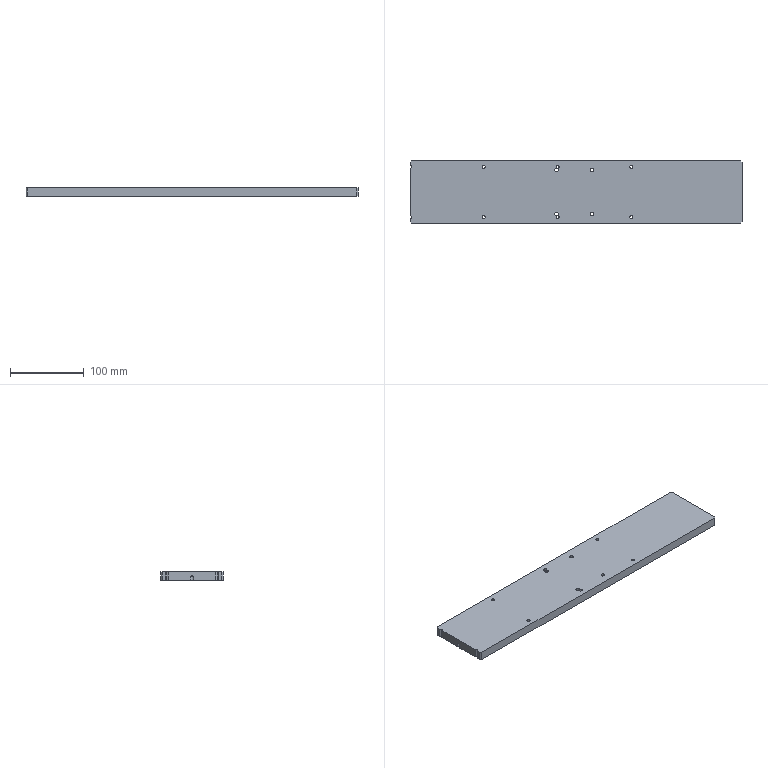Part | SolidWorks | features BaseBody 1 | 1 solid | 46 faces | box 450 x 85 x 12 mm | volume 456645 mm3 | cylinder 31 | plane 12 | cone 3 | commonest cylinder face diameters 4.2 x18 5 x13
STEP:
#1=CARTESIAN_POINT('',(-225.,-40.5,12.));
#2=VERTEX_POINT('',#1);
#3=CARTESIAN_POINT('',(-223.,-42.5,12.));
#4=VERTEX_POINT('',#3);
#5=CARTESIAN_POINT('',(-223.,-42.5,12.));
#6=DIRECTION('',(0.7071,-0.7071,0.));
#7=VECTOR('',#6,1000.);
#8=LINE('',#5,#7);
#9=EDGE_CURVE('',#2,#4,#8,.T.);
#10=ORIENTED_EDGE('',*,*,#9,.F.);
#11=CARTESIAN_POINT('',(-225.,-40.5,0.));
#12=VERTEX_POINT('',#11);
#13=CARTESIAN_POINT('',(-225.,-40.5,12.));
#14=DIRECTION('',(0.,0.,1.));
#15=VECTOR('',#14,1000.);
#16=LINE('',#13,#15);
#17=EDGE_CURVE('',#12,#2,#16,.T.);
#18=ORIENTED_EDGE('',*,*,#17,.F.);
#19=CARTESIAN_POINT('',(-223.,-42.5,0.));
#20=VERTEX_POINT('',#19);
#21=CARTESIAN_POINT('',(-132.75,-132.75,0.));
#22=DIRECTION('',(-0.7071,0.7071,0.));
#23=VECTOR('',#22,1000.);
#24=LINE('',#21,#23);
#25=EDGE_CURVE('',#20,#12,#24,.T.);
#26=ORIENTED_EDGE('',*,*,#25,.F.);
#27=CARTESIAN_POINT('',(-223.,-42.5,12.));
#28=DIRECTION('',(0.,0.,-1.));
#29=VECTOR('',#28,1000.);
#30=LINE('',#27,#29);
#31=EDGE_CURVE('',#4,#20,#30,.T.);
#32=ORIENTED_EDGE('',*,*,#31,.F.);
#33=EDGE_LOOP('',(#10,#18,#26,#32));
#34=FACE_OUTER_BOUND('',#33,.T.);
#35=CARTESIAN_POINT('',(-223.,-42.5,12.));
#36=DIRECTION('',(0.7071,0.7071,0.));
#37=DIRECTION('',(0.,0.,-1.));
#38=AXIS2_PLACEMENT_3D('',#35,#36,#37);
#39=PLANE('',#38);
#40=ADVANCED_FACE('',(#34),#39,.F.);
#41=CARTESIAN_POINT('',(-223.,42.5,12.));
#42=VERTEX_POINT('',#41);
#43=CARTESIAN_POINT('',(-225.,40.5,12.));
#44=VERTEX_POINT('',#43);
#45=CARTESIAN_POINT('',(-225.,40.5,12.));
#46=DIRECTION('',(-0.7071,-0.7071,0.));
#47=VECTOR('',#46,1000.);
#48=LINE('',#45,#47);
#49=EDGE_CURVE('',#42,#44,#48,.T.);
#50=ORIENTED_EDGE('',*,*,#49,.F.);
#51=CARTESIAN_POINT('',(-223.,42.5,0.));
#52=VERTEX_POINT('',#51);
#53=CARTESIAN_POINT('',(-223.,42.5,12.));
#54=DIRECTION('',(0.,0.,1.));
#55=VECTOR('',#54,1000.);
#56=LINE('',#53,#55);
#57=EDGE_CURVE('',#52,#42,#56,.T.);
#58=ORIENTED_EDGE('',*,*,#57,.F.);
#59=CARTESIAN_POINT('',(-225.,40.5,0.));
#60=VERTEX_POINT('',#59);
#61=CARTESIAN_POINT('',(-132.75,132.75,0.));
#62=DIRECTION('',(0.7071,0.7071,0.));
#63=VECTOR('',#62,1000.);
#64=LINE('',#61,#63);
#65=EDGE_CURVE('',#60,#52,#64,.T.);
#66=ORIENTED_EDGE('',*,*,#65,.F.);
#67=CARTESIAN_POINT('',(-225.,40.5,12.));
#68=DIRECTION('',(0.,0.,-1.));
#69=VECTOR('',#68,1000.);
#70=LINE('',#67,#69);
#71=EDGE_CURVE('',#44,#60,#70,.T.);
#72=ORIENTED_EDGE('',*,*,#71,.F.);
#73=EDGE_LOOP('',(#50,#58,#66,#72));
#74=FACE_OUTER_BOUND('',#73,.T.);
#75=CARTESIAN_POINT('',(-225.,40.5,12.));
#76=DIRECTION('',(0.7071,-0.7071,0.));
#77=DIRECTION('',(0.,0.,-1.));
#78=AXIS2_PLACEMENT_3D('',#75,#76,#77);
#79=PLANE('',#78);
#80=ADVANCED_FACE('',(#74),#79,.F.);
#81=CARTESIAN_POINT('',(223.,-42.5,12.));
#82=VERTEX_POINT('',#81);
#83=CARTESIAN_POINT('',(225.,-40.5,12.));
#84=VERTEX_POINT('',#83);
#85=CARTESIAN_POINT('',(225.,-40.5,12.));
#86=DIRECTION('',(0.7071,0.7071,0.));
#87=VECTOR('',#86,1000.);
#88=LINE('',#85,#87);
#89=EDGE_CURVE('',#82,#84,#88,.T.);
#90=ORIENTED_EDGE('',*,*,#89,.F.);
#91=CARTESIAN_POINT('',(223.,-42.5,0.));
#92=VERTEX_POINT('',#91);
#93=CARTESIAN_POINT('',(223.,-42.5,12.));
#94=DIRECTION('',(0.,0.,1.));
#95=VECTOR('',#94,1000.);
#96=LINE('',#93,#95);
#97=EDGE_CURVE('',#92,#82,#96,.T.);
#98=ORIENTED_EDGE('',*,*,#97,.F.);
#99=CARTESIAN_POINT('',(225.,-40.5,0.));
#100=VERTEX_POINT('',#99);
#101=CARTESIAN_POINT('',(132.75,-132.75,0.));
#102=DIRECTION('',(-0.7071,-0.7071,0.));
#103=VECTOR('',#102,1000.);
#104=LINE('',#101,#103);
#105=EDGE_CURVE('',#100,#92,#104,.T.);
#106=ORIENTED_EDGE('',*,*,#105,.F.);
#107=CARTESIAN_POINT('',(225.,-40.5,12.));
#108=DIRECTION('',(0.,0.,-1.));
#109=VECTOR('',#108,1000.);
#110=LINE('',#107,#109);
#111=EDGE_CURVE('',#84,#100,#110,.T.);
#112=ORIENTED_EDGE('',*,*,#111,.F.);
#113=EDGE_LOOP('',(#90,#98,#106,#112));
#114=FACE_OUTER_BOUND('',#113,.T.);
#115=CARTESIAN_POINT('',(225.,-40.5,12.));
#116=DIRECTION('',(-0.7071,0.7071,0.));
#117=DIRECTION('',(0.,0.,1.));
#118=AXIS2_PLACEMENT_3D('',#115,#116,#117);
#119=PLANE('',#118);
#120=ADVANCED_FACE('',(#114),#119,.F.);
#121=CARTESIAN_POINT('',(225.,40.5,12.));
#122=VERTEX_POINT('',#121);
#123=CARTESIAN_POINT('',(223.,42.5,12.));
#124=VERTEX_POINT('',#123);
#125=CARTESIAN_POINT('',(223.,42.5,12.));
#126=DIRECTION('',(-0.7071,0.7071,0.));
#127=VECTOR('',#126,1000.);
#128=LINE('',#125,#127);
#129=EDGE_CURVE('',#122,#124,#128,.T.);
#130=ORIENTED_EDGE('',*,*,#129,.F.);
#131=CARTESIAN_POINT('',(225.,40.5,0.));
#132=VERTEX_POINT('',#131);
#133=CARTESIAN_POINT('',(225.,40.5,12.));
#134=DIRECTION('',(0.,0.,1.));
#135=VECTOR('',#134,1000.);
#136=LINE('',#133,#135);
#137=EDGE_CURVE('',#132,#122,#136,.T.);
#138=ORIENTED_EDGE('',*,*,#137,.F.);
#139=CARTESIAN_POINT('',(223.,42.5,0.));
#140=VERTEX_POINT('',#139);
#141=CARTESIAN_POINT('',(132.75,132.75,0.));
#142=DIRECTION('',(0.7071,-0.7071,0.));
#143=VECTOR('',#142,1000.);
#144=LINE('',#141,#143);
#145=EDGE_CURVE('',#140,#132,#144,.T.);
#146=ORIENTED_EDGE('',*,*,#145,.F.);
#147=CARTESIAN_POINT('',(223.,42.5,12.));
#148=DIRECTION('',(0.,0.,-1.));
#149=VECTOR('',#148,1000.);
#150=LINE('',#147,#149);
#151=EDGE_CURVE('',#124,#140,#150,.T.);
#152=ORIENTED_EDGE('',*,*,#151,.F.);
#153=EDGE_LOOP('',(#130,#138,#146,#152));
#154=FACE_OUTER_BOUND('',#153,.T.);
#155=CARTESIAN_POINT('',(223.,42.5,12.));
#156=DIRECTION('',(-0.7071,-0.7071,0.));
#157=DIRECTION('',(-0.7071,0.7071,0.));
#158=AXIS2_PLACEMENT_3D('',#155,#156,#157);
#159=PLANE('',#158);
#160=ADVANCED_FACE('',(#154),#159,.F.);
#161=CARTESIAN_POINT('',(77.5,0.,5.));
#162=VERTEX_POINT('',#161);
#163=CARTESIAN_POINT('',(77.5,0.,0.));
#164=VERTEX_POINT('',#163);
#165=CARTESIAN_POINT('',(77.5,0.,0.));
#166=DIRECTION('',(0.,0.,-1.));
#167=VECTOR('',#166,1000.);
#168=LINE('',#165,#167);
#169=EDGE_CURVE('',#162,#164,#168,.T.);
#170=ORIENTED_EDGE('',*,*,#169,.F.);
#171=CARTESIAN_POINT('',(72.5,0.,5.));
#172=VERTEX_POINT('',#171);
#173=CARTESIAN_POINT('',(75.,0.,5.));
#174=DIRECTION('',(0.,0.,-1.));
#175=DIRECTION('',(-1.,0.,0.));
#176=AXIS2_PLACEMENT_3D('',#173,#174,#175);
#177=CIRCLE('',#176,2.5);
#178=EDGE_CURVE('',#172,#162,#177,.T.);
#179=ORIENTED_EDGE('',*,*,#178,.F.);
#180=CARTESIAN_POINT('',(72.5,0.,0.));
#181=VERTEX_POINT('',#180);
#182=CARTESIAN_POINT('',(72.5,0.,0.));
#183=DIRECTION('',(0.,0.,-1.));
#184=VECTOR('',#183,1000.);
#185=LINE('',#182,#184);
#186=EDGE_CURVE('',#172,#181,#185,.T.);
#187=ORIENTED_EDGE('',*,*,#186,.T.);
#188=CARTESIAN_POINT('',(75.,0.,0.));
#189=DIRECTION('',(0.,0.,-1.));
#190=DIRECTION('',(-1.,0.,0.));
#191=AXIS2_PLACEMENT_3D('',#188,#189,#190);
#192=CIRCLE('',#191,2.5);
#193=EDGE_CURVE('',#181,#164,#192,.T.);
#194=ORIENTED_EDGE('',*,*,#193,.T.);
#195=EDGE_LOOP('',(#170,#179,#187,#194));
#196=FACE_OUTER_BOUND('',#195,.T.);
#197=CARTESIAN_POINT('',(75.,0.,0.));
#198=DIRECTION('',(0.,0.,-1.));
#199=DIRECTION('',(-1.,0.,0.));
#200=AXIS2_PLACEMENT_3D('',#197,#198,#199);
#201=CYLINDRICAL_SURFACE('',#200,2.5);
#202=ADVANCED_FACE('',(#196),#201,.F.);
#203=CARTESIAN_POINT('',(75.,0.,6.502));
#204=VERTEX_POINT('',#203);
#205=CARTESIAN_POINT('',(77.5,0.,5.));
#206=DIRECTION('',(0.8572,0.,-0.515));
#207=VECTOR('',#206,1000.);
#208=LINE('',#205,#207);
#209=EDGE_CURVE('',#204,#162,#208,.T.);
#210=ORIENTED_EDGE('',*,*,#209,.F.);
#211=CARTESIAN_POINT('',(72.5,0.,5.));
#212=DIRECTION('',(-0.8572,0.,-0.515));
#213=VECTOR('',#212,1000.);
#214=LINE('',#211,#213);
#215=EDGE_CURVE('',#204,#172,#214,.T.);
#216=ORIENTED_EDGE('',*,*,#215,.T.);
#217=ORIENTED_EDGE('',*,*,#178,.T.);
#218=EDGE_LOOP('',(#210,#216,#217));
#219=FACE_OUTER_BOUND('',#218,.T.);
#220=CARTESIAN_POINT('',(75.,0.,5.));
#221=DIRECTION('',(0.,0.,-1.));
#222=DIRECTION('',(-1.,0.,0.));
#223=AXIS2_PLACEMENT_3D('',#220,#221,#222);
#224=CONICAL_SURFACE('',#223,2.5,1.03);
#225=ADVANCED_FACE('',(#219),#224,.F.);
#226=CARTESIAN_POINT('',(-225.,2.5,5.));
#227=VERTEX_POINT('',#226);
#228=CARTESIAN_POINT('',(-225.,0.,6.502));
#229=VERTEX_POINT('',#228);
#230=CARTESIAN_POINT('',(-225.,0.,6.502));
#231=DIRECTION('',(0.,-0.8572,0.515));
#232=VECTOR('',#231,1000.);
#233=LINE('',#230,#232);
#234=EDGE_CURVE('',#227,#229,#233,.T.);
#235=ORIENTED_EDGE('',*,*,#234,.F.);
#236=CARTESIAN_POINT('',(-225.,-2.5,5.));
#237=VERTEX_POINT('',#236);
#238=CARTESIAN_POINT('',(-225.,0.,5.));
#239=DIRECTION('',(0.,0.,-1.));
#240=DIRECTION('',(-1.,0.,0.));
#241=AXIS2_PLACEMENT_3D('',#238,#239,#240);
#242=CIRCLE('',#241,2.5);
#243=EDGE_CURVE('',#227,#237,#242,.T.);
#244=ORIENTED_EDGE('',*,*,#243,.T.);
#245=CARTESIAN_POINT('',(-225.,0.,6.502));
#246=DIRECTION('',(0.,-0.8572,-0.515));
#247=VECTOR('',#246,1000.);
#248=LINE('',#245,#247);
#249=EDGE_CURVE('',#229,#237,#248,.T.);
#250=ORIENTED_EDGE('',*,*,#249,.F.);
#251=EDGE_LOOP('',(#235,#244,#250));
#252=FACE_OUTER_BOUND('',#251,.T.);
#253=CARTESIAN_POINT('',(-225.,0.,5.));
#254=DIRECTION('',(0.,0.,-1.));
#255=DIRECTION('',(-1.,0.,0.));
#256=AXIS2_PLACEMENT_3D('',#253,#254,#255);
#257=CONICAL_SURFACE('',#256,2.5,1.03);
#258=ADVANCED_FACE('',(#252),#257,.F.);
#259=ORIENTED_EDGE('',*,*,#243,.F.);
#260=CARTESIAN_POINT('',(-225.,2.5,0.));
#261=VERTEX_POINT('',#260);
#262=CARTESIAN_POINT('',(-225.,2.5,0.));
#263=DIRECTION('',(0.,0.,1.));
#264=VECTOR('',#263,1000.);
#265=LINE('',#262,#264);
#266=EDGE_CURVE('',#261,#227,#265,.T.);
#267=ORIENTED_EDGE('',*,*,#266,.F.);
#268=CARTESIAN_POINT('',(-225.,-2.5,0.));
#269=VERTEX_POINT('',#268);
#270=CARTESIAN_POINT('',(-225.,0.,0.));
#271=DIRECTION('',(0.,0.,-1.));
#272=DIRECTION('',(-1.,0.,0.));
#273=AXIS2_PLACEMENT_3D('',#270,#271,#272);
#274=CIRCLE('',#273,2.5);
#275=EDGE_CURVE('',#261,#269,#274,.T.);
#276=ORIENTED_EDGE('',*,*,#275,.T.);
#277=CARTESIAN_POINT('',(-225.,-2.5,0.));
#278=DIRECTION('',(0.,0.,-1.));
#279=VECTOR('',#278,1000.);
#280=LINE('',#277,#279);
#281=EDGE_CURVE('',#237,#269,#280,.T.);
#282=ORIENTED_EDGE('',*,*,#281,.F.);
#283=EDGE_LOOP('',(#259,#267,#276,#282));
#284=FACE_OUTER_BOUND('',#283,.T.);
#285=CARTESIAN_POINT('',(-225.,0.,0.));
#286=DIRECTION('',(0.,0.,-1.));
#287=DIRECTION('',(-1.,0.,0.));
#288=AXIS2_PLACEMENT_3D('',#285,#286,#287);
#289=CYLINDRICAL_SURFACE('',#288,2.5);
#290=ADVANCED_FACE('',(#284),#289,.F.);
#291=CARTESIAN_POINT('',(72.9,34.,0.));
#292=VERTEX_POINT('',#291);
#293=CARTESIAN_POINT('',(72.9,34.,12.));
#294=VERTEX_POINT('',#293);
#295=CARTESIAN_POINT('',(72.9,34.,12.));
#296=DIRECTION('',(0.,0.,1.));
#297=VECTOR('',#296,1000.);
#298=LINE('',#295,#297);
#299=EDGE_CURVE('',#292,#294,#298,.T.);
#300=ORIENTED_EDGE('',*,*,#299,.F.);
#301=CARTESIAN_POINT('',(77.1,34.,0.));
#302=VERTEX_POINT('',#301);
#303=CARTESIAN_POINT('',(75.,34.,0.));
#304=DIRECTION('',(0.,0.,1.));
#305=DIRECTION('',(1.,0.,0.));
#306=AXIS2_PLACEMENT_3D('',#303,#304,#305);
#307=CIRCLE('',#306,2.1);
#308=EDGE_CURVE('',#302,#292,#307,.T.);
#309=ORIENTED_EDGE('',*,*,#308,.F.);
#310=CARTESIAN_POINT('',(77.1,34.,12.));
#311=VERTEX_POINT('',#310);
#312=CARTESIAN_POINT('',(77.1,34.,12.));
#313=DIRECTION('',(0.,0.,1.));
#314=VECTOR('',#313,1000.);
#315=LINE('',#312,#314);
#316=EDGE_CURVE('',#302,#311,#315,.T.);
#317=ORIENTED_EDGE('',*,*,#316,.T.);
#318=CARTESIAN_POINT('',(75.,34.,12.));
#319=DIRECTION('',(0.,0.,1.));
#320=DIRECTION('',(1.,0.,0.));
#321=AXIS2_PLACEMENT_3D('',#318,#319,#320);
#322=CIRCLE('',#321,2.1);
#323=EDGE_CURVE('',#311,#294,#322,.T.);
#324=ORIENTED_EDGE('',*,*,#323,.T.);
#325=EDGE_LOOP('',(#300,#309,#317,#324));
#326=FACE_OUTER_BOUND('',#325,.T.);
#327=CARTESIAN_POINT('',(75.,34.,12.));
#328=DIRECTION('',(0.,0.,1.));
#329=DIRECTION('',(1.,0.,0.));
#330=AXIS2_PLACEMENT_3D('',#327,#328,#329);
#331=CYLINDRICAL_SURFACE('',#330,2.1);
#332=ADVANCED_FACE('',(#326),#331,.F.);
#333=CARTESIAN_POINT('',(72.9,-34.,0.));
#334=VERTEX_POINT('',#333);
#335=CARTESIAN_POINT('',(72.9,-34.,12.));
#336=VERTEX_POINT('',#335);
#337=CARTESIAN_POINT('',(72.9,-34.,12.));
#338=DIRECTION('',(0.,0.,1.));
#339=VECTOR('',#338,1000.);
#340=LINE('',#337,#339);
#341=EDGE_CURVE('',#334,#336,#340,.T.);
#342=ORIENTED_EDGE('',*,*,#341,.F.);
#343=CARTESIAN_POINT('',(77.1,-34.,0.));
#344=VERTEX_POINT('',#343);
#345=CARTESIAN_POINT('',(75.,-34.,0.));
#346=DIRECTION('',(0.,0.,1.));
#347=DIRECTION('',(1.,0.,0.));
#348=AXIS2_PLACEMENT_3D('',#345,#346,#347);
#349=CIRCLE('',#348,2.1);
#350=EDGE_CURVE('',#344,#334,#349,.T.);
#351=ORIENTED_EDGE('',*,*,#350,.F.);
#352=CARTESIAN_POINT('',(77.1,-34.,12.));
#353=VERTEX_POINT('',#352);
#354=CARTESIAN_POINT('',(77.1,-34.,12.));
#355=DIRECTION('',(0.,0.,1.));
#356=VECTOR('',#355,1000.);
#357=LINE('',#354,#356);
#358=EDGE_CURVE('',#344,#353,#357,.T.);
#359=ORIENTED_EDGE('',*,*,#358,.T.);
#360=CARTESIAN_POINT('',(75.,-34.,12.));
#361=DIRECTION('',(0.,0.,1.));
#362=DIRECTION('',(1.,0.,0.));
#363=AXIS2_PLACEMENT_3D('',#360,#361,#362);
#364=CIRCLE('',#363,2.1);
#365=EDGE_CURVE('',#353,#336,#364,.T.);
#366=ORIENTED_EDGE('',*,*,#365,.T.);
#367=EDGE_LOOP('',(#342,#351,#359,#366));
#368=FACE_OUTER_BOUND('',#367,.T.);
#369=CARTESIAN_POINT('',(75.,-34.,12.));
#370=DIRECTION('',(0.,0.,1.));
#371=DIRECTION('',(1.,0.,0.));
#372=AXIS2_PLACEMENT_3D('',#369,#370,#371);
#373=CYLINDRICAL_SURFACE('',#372,2.1);
#374=ADVANCED_FACE('',(#368),#373,.F.);
#375=CARTESIAN_POINT('',(-22.9,34.,0.));
#376=VERTEX_POINT('',#375);
#377=CARTESIAN_POINT('',(-22.9,34.,12.));
#378=VERTEX_POINT('',#377);
#379=CARTESIAN_POINT('',(-22.9,34.,12.));
#380=DIRECTION('',(0.,0.,1.));
#381=VECTOR('',#380,1000.);
#382=LINE('',#379,#381);
#383=EDGE_CURVE('',#376,#378,#382,.T.);
#384=ORIENTED_EDGE('',*,*,#383,.F.);
#385=CARTESIAN_POINT('',(-24.879,31.903,0.));
#386=VERTEX_POINT('',#385);
#387=CARTESIAN_POINT('',(-25.,34.,0.));
#388=DIRECTION('',(0.,0.,-1.));
#389=DIRECTION('',(-1.,0.,0.));
#390=AXIS2_PLACEMENT_3D('',#387,#388,#389);
#391=CIRCLE('',#390,2.1);
#392=EDGE_CURVE('',#376,#386,#391,.T.);
#393=ORIENTED_EDGE('',*,*,#392,.T.);
#394=CARTESIAN_POINT('',(-24.879,31.903,12.));
#395=VERTEX_POINT('',#394);
#396=CARTESIAN_POINT('',(-24.879,31.903,6.));
#397=DIRECTION('',(0.,0.,-1.));
#398=VECTOR('',#397,1000.);
#399=LINE('',#396,#398);
#400=EDGE_CURVE('',#395,#386,#399,.T.);
#401=ORIENTED_EDGE('',*,*,#400,.F.);
#402=CARTESIAN_POINT('',(-25.,34.,12.));
#403=DIRECTION('',(0.,0.,1.));
#404=DIRECTION('',(1.,0.,0.));
#405=AXIS2_PLACEMENT_3D('',#402,#403,#404);
#406=CIRCLE('',#405,2.1);
#407=EDGE_CURVE('',#395,#378,#406,.T.);
#408=ORIENTED_EDGE('',*,*,#407,.T.);
#409=EDGE_LOOP('',(#384,#393,#401,#408));
#410=FACE_OUTER_BOUND('',#409,.T.);
#411=CARTESIAN_POINT('',(-25.,34.,12.));
#412=DIRECTION('',(0.,0.,1.));
#413=DIRECTION('',(1.,0.,0.));
#414=AXIS2_PLACEMENT_3D('',#411,#412,#413);
#415=CYLINDRICAL_SURFACE('',#414,2.1);
#416=ADVANCED_FACE('',(#410),#415,.F.);
#417=CARTESIAN_POINT('',(-27.1,-34.,0.));
#418=VERTEX_POINT('',#417);
#419=CARTESIAN_POINT('',(-27.1,-34.,12.));
#420=VERTEX_POINT('',#419);
#421=CARTESIAN_POINT('',(-27.1,-34.,12.));
#422=DIRECTION('',(0.,0.,1.));
#423=VECTOR('',#422,1000.);
#424=LINE('',#421,#423);
#425=EDGE_CURVE('',#418,#420,#424,.T.);
#426=ORIENTED_EDGE('',*,*,#425,.F.);
#427=CARTESIAN_POINT('',(-26.47,-32.5,0.));
#428=VERTEX_POINT('',#427);
#429=CARTESIAN_POINT('',(-25.,-34.,0.));
#430=DIRECTION('',(0.,0.,1.));
#431=DIRECTION('',(1.,0.,0.));
#432=AXIS2_PLACEMENT_3D('',#429,#430,#431);
#433=CIRCLE('',#432,2.1);
#434=EDGE_CURVE('',#428,#418,#433,.T.);
#435=ORIENTED_EDGE('',*,*,#434,.F.);
#436=CARTESIAN_POINT('',(-26.47,-32.5,12.));
#437=VERTEX_POINT('',#436);
#438=CARTESIAN_POINT('',(-26.47,-32.5,6.));
#439=DIRECTION('',(0.,0.,-1.));
#440=VECTOR('',#439,1000.);
#441=LINE('',#438,#440);
#442=EDGE_CURVE('',#437,#428,#441,.T.);
#443=ORIENTED_EDGE('',*,*,#442,.F.);
#444=CARTESIAN_POINT('',(-25.,-34.,12.));
#445=DIRECTION('',(0.,0.,1.));
#446=DIRECTION('',(1.,0.,0.));
#447=AXIS2_PLACEMENT_3D('',#444,#445,#446);
#448=CIRCLE('',#447,2.1);
#449=EDGE_CURVE('',#437,#420,#448,.T.);
#450=ORIENTED_EDGE('',*,*,#449,.T.);
#451=EDGE_LOOP('',(#426,#435,#443,#450));
#452=FACE_OUTER_BOUND('',#451,.T.);
#453=CARTESIAN_POINT('',(-25.,-34.,12.));
#454=DIRECTION('',(0.,0.,1.));
#455=DIRECTION('',(1.,0.,0.));
#456=AXIS2_PLACEMENT_3D('',#453,#454,#455);
#457=CYLINDRICAL_SURFACE('',#456,2.1);
#458=ADVANCED_FACE('',(#452),#457,.F.);
#459=CARTESIAN_POINT('',(-127.1,34.,0.));
#460=VERTEX_POINT('',#459);
#461=CARTESIAN_POINT('',(-127.1,34.,12.));
#462=VERTEX_POINT('',#461);
#463=CARTESIAN_POINT('',(-127.1,34.,12.));
#464=DIRECTION('',(0.,0.,1.));
#465=VECTOR('',#464,1000.);
#466=LINE('',#463,#465);
#467=EDGE_CURVE('',#460,#462,#466,.T.);
#468=ORIENTED_EDGE('',*,*,#467,.F.);
#469=CARTESIAN_POINT('',(-122.9,34.,0.));
#470=VERTEX_POINT('',#469);
#471=CARTESIAN_POINT('',(-125.,34.,0.));
#472=DIRECTION('',(0.,0.,1.));
#473=DIRECTION('',(1.,0.,0.));
#474=AXIS2_PLACEMENT_3D('',#471,#472,#473);
#475=CIRCLE('',#474,2.1);
#476=EDGE_CURVE('',#470,#460,#475,.T.);
#477=ORIENTED_EDGE('',*,*,#476,.F.);
#478=CARTESIAN_POINT('',(-122.9,34.,12.));
#479=VERTEX_POINT('',#478);
#480=CARTESIAN_POINT('',(-122.9,34.,12.));
#481=DIRECTION('',(0.,0.,1.));
#482=VECTOR('',#481,1000.);
#483=LINE('',#480,#482);
#484=EDGE_CURVE('',#470,#479,#483,.T.);
#485=ORIENTED_EDGE('',*,*,#484,.T.);
#486=CARTESIAN_POINT('',(-125.,34.,12.));
#487=DIRECTION('',(0.,0.,1.));
#488=DIRECTION('',(1.,0.,0.));
#489=AXIS2_PLACEMENT_3D('',#486,#487,#488);
#490=CIRCLE('',#489,2.1);
#491=EDGE_CURVE('',#479,#462,#490,.T.);
#492=ORIENTED_EDGE('',*,*,#491,.T.);
#493=EDGE_LOOP('',(#468,#477,#485,#492));
#494=FACE_OUTER_BOUND('',#493,.T.);
#495=CARTESIAN_POINT('',(-125.,34.,12.));
#496=DIRECTION('',(0.,0.,1.));
#497=DIRECTION('',(1.,0.,0.));
#498=AXIS2_PLACEMENT_3D('',#495,#496,#497);
#499=CYLINDRICAL_SURFACE('',#498,2.1);
#500=ADVANCED_FACE('',(#494),#499,.F.);
#501=CARTESIAN_POINT('',(-127.1,-34.,0.));
#502=VERTEX_POINT('',#501);
#503=CARTESIAN_POINT('',(-127.1,-34.,12.));
#504=VERTEX_POINT('',#503);
#505=CARTESIAN_POINT('',(-127.1,-34.,12.));
#506=DIRECTION('',(0.,0.,1.));
#507=VECTOR('',#506,1000.);
#508=LINE('',#505,#507);
#509=EDGE_CURVE('',#502,#504,#508,.T.);
#510=ORIENTED_EDGE('',*,*,#509,.F.);
#511=CARTESIAN_POINT('',(-122.9,-34.,0.));
#512=VERTEX_POINT('',#511);
#513=CARTESIAN_POINT('',(-125.,-34.,0.));
#514=DIRECTION('',(0.,0.,1.));
#515=DIRECTION('',(1.,0.,0.));
#516=AXIS2_PLACEMENT_3D('',#513,#514,#515);
#517=CIRCLE('',#516,2.1);
#518=EDGE_CURVE('',#512,#502,#517,.T.);
#519=ORIENTED_EDGE('',*,*,#518,.F.);
#520=CARTESIAN_POINT('',(-122.9,-34.,12.));
#521=VERTEX_POINT('',#520);
#522=CARTESIAN_POINT('',(-122.9,-34.,12.));
#523=DIRECTION('',(0.,0.,1.));
#524=VECTOR('',#523,1000.);
#525=LINE('',#522,#524);
#526=EDGE_CURVE('',#512,#521,#525,.T.);
#527=ORIENTED_EDGE('',*,*,#526,.T.);
#528=CARTESIAN_POINT('',(-125.,-34.,12.));
#529=DIRECTION('',(0.,0.,1.));
#530=DIRECTION('',(1.,0.,0.));
#531=AXIS2_PLACEMENT_3D('',#528,#529,#530);
#532=CIRCLE('',#531,2.1);
#533=EDGE_CURVE('',#521,#504,#532,.T.);
#534=ORIENTED_EDGE('',*,*,#533,.T.);
#535=EDGE_LOOP('',(#510,#519,#527,#534));
#536=FACE_OUTER_BOUND('',#535,.T.);
#537=CARTESIAN_POINT('',(-125.,-34.,12.));
#538=DIRECTION('',(0.,0.,1.));
#539=DIRECTION('',(1.,0.,0.));
#540=AXIS2_PLACEMENT_3D('',#537,#538,#539);
#541=CYLINDRICAL_SURFACE('',#540,2.1);
#542=ADVANCED_FACE('',(#536),#541,.F.);
#543=CARTESIAN_POINT('',(-222.9,34.,0.));
#544=VERTEX_POINT('',#543);
#545=CARTESIAN_POINT('',(-222.9,34.,12.));
#546=VERTEX_POINT('',#545);
#547=CARTESIAN_POINT('',(-222.9,34.,12.));
#548=DIRECTION('',(0.,0.,1.));
#549=VECTOR('',#548,1000.);
#550=LINE('',#547,#549);
#551=EDGE_CURVE('',#544,#546,#550,.T.);
#552=ORIENTED_EDGE('',*,*,#551,.F.);
#553=CARTESIAN_POINT('',(-225.,31.9,0.));
#554=VERTEX_POINT('',#553);
#555=CARTESIAN_POINT('',(-225.,34.,0.));
#556=DIRECTION('',(0.,0.,1.));
#557=DIRECTION('',(1.,0.,0.));
#558=AXIS2_PLACEMENT_3D('',#555,#556,#557);
#559=CIRCLE('',#558,2.1);
#560=EDGE_CURVE('',#554,#544,#559,.T.);
#561=ORIENTED_EDGE('',*,*,#560,.F.);
#562=CARTESIAN_POINT('',(-225.,31.9,12.));
#563=VERTEX_POINT('',#562);
#564=CARTESIAN_POINT('',(-225.,31.9,12.));
#565=DIRECTION('',(0.,0.,-1.));
#566=VECTOR('',#565,1000.);
#567=LINE('',#564,#566);
#568=EDGE_CURVE('',#563,#554,#567,.T.);
#569=ORIENTED_EDGE('',*,*,#568,.F.);
#570=CARTESIAN_POINT('',(-225.,34.,12.));
#571=DIRECTION('',(0.,0.,1.));
#572=DIRECTION('',(1.,0.,0.));
#573=AXIS2_PLACEMENT_3D('',#570,#571,#572);
#574=CIRCLE('',#573,2.1);
#575=EDGE_CURVE('',#563,#546,#574,.T.);
#576=ORIENTED_EDGE('',*,*,#575,.T.);
#577=EDGE_LOOP('',(#552,#561,#569,#576));
#578=FACE_OUTER_BOUND('',#577,.T.);
#579=CARTESIAN_POINT('',(-225.,34.,12.));
#580=DIRECTION('',(0.,0.,1.));
#581=DIRECTION('',(1.,0.,0.));
#582=AXIS2_PLACEMENT_3D('',#579,#580,#581);
#583=CYLINDRICAL_SURFACE('',#582,2.1);
#584=ADVANCED_FACE('',(#578),#583,.F.);
#585=CARTESIAN_POINT('',(-222.9,-34.,0.));
#586=VERTEX_POINT('',#585);
#587=CARTESIAN_POINT('',(-222.9,-34.,12.));
#588=VERTEX_POINT('',#587);
#589=CARTESIAN_POINT('',(-222.9,-34.,12.));
#590=DIRECTION('',(0.,0.,1.));
#591=VECTOR('',#590,1000.);
#592=LINE('',#589,#591);
#593=EDGE_CURVE('',#586,#588,#592,.T.);
#594=ORIENTED_EDGE('',*,*,#593,.F.);
#595=CARTESIAN_POINT('',(-225.,-36.1,0.));
#596=VERTEX_POINT('',#595);
#597=CARTESIAN_POINT('',(-225.,-34.,0.));
#598=DIRECTION('',(0.,0.,-1.));
#599=DIRECTION('',(-1.,0.,0.));
#600=AXIS2_PLACEMENT_3D('',#597,#598,#599);
#601=CIRCLE('',#600,2.1);
#602=EDGE_CURVE('',#586,#596,#601,.T.);
#603=ORIENTED_EDGE('',*,*,#602,.T.);
#604=CARTESIAN_POINT('',(-225.,-36.1,12.));
#605=VERTEX_POINT('',#604);
#606=CARTESIAN_POINT('',(-225.,-36.1,12.));
#607=DIRECTION('',(0.,0.,-1.));
#608=VECTOR('',#607,1000.);
#609=LINE('',#606,#608);
#610=EDGE_CURVE('',#605,#596,#609,.T.);
#611=ORIENTED_EDGE('',*,*,#610,.F.);
#612=CARTESIAN_POINT('',(-225.,-34.,12.));
#613=DIRECTION('',(0.,0.,1.));
#614=DIRECTION('',(1.,0.,0.));
#615=AXIS2_PLACEMENT_3D('',#612,#613,#614);
#616=CIRCLE('',#615,2.1);
#617=EDGE_CURVE('',#605,#588,#616,.T.);
#618=ORIENTED_EDGE('',*,*,#617,.T.);
#619=EDGE_LOOP('',(#594,#603,#611,#618));
#620=FACE_OUTER_BOUND('',#619,.T.);
#621=CARTESIAN_POINT('',(-225.,-34.,12.));
#622=DIRECTION('',(0.,0.,1.));
#623=DIRECTION('',(1.,0.,0.));
#624=AXIS2_PLACEMENT_3D('',#621,#622,#623);
#625=CYLINDRICAL_SURFACE('',#624,2.1);
#626=ADVANCED_FACE('',(#620),#625,.F.);
#627=CARTESIAN_POINT('',(-24.,30.,12.));
#628=VERTEX_POINT('',#627);
#629=CARTESIAN_POINT('',(-24.,30.,0.));
#630=VERTEX_POINT('',#629);
#631=CARTESIAN_POINT('',(-24.,30.,0.));
#632=DIRECTION('',(0.,0.,-1.));
#633=VECTOR('',#632,1000.);
#634=LINE('',#631,#633);
#635=EDGE_CURVE('',#628,#630,#634,.T.);
#636=ORIENTED_EDGE('',*,*,#635,.F.);
#637=CARTESIAN_POINT('',(-26.5,30.,12.));
#638=DIRECTION('',(0.,0.,-1.));
#639=DIRECTION('',(-1.,0.,0.));
#640=AXIS2_PLACEMENT_3D('',#637,#638,#639);
#641=CIRCLE('',#640,2.5);
#642=EDGE_CURVE('',#395,#628,#641,.T.);
#643=ORIENTED_EDGE('',*,*,#642,.F.);
#644=ORIENTED_EDGE('',*,*,#400,.T.);
#645=CARTESIAN_POINT('',(-26.5,30.,0.));
#646=DIRECTION('',(0.,0.,-1.));
#647=DIRECTION('',(-1.,0.,0.));
#648=AXIS2_PLACEMENT_3D('',#645,#646,#647);
#649=CIRCLE('',#648,2.5);
#650=EDGE_CURVE('',#386,#630,#649,.T.);
#651=ORIENTED_EDGE('',*,*,#650,.T.);
#652=EDGE_LOOP('',(#636,#643,#644,#651));
#653=FACE_OUTER_BOUND('',#652,.T.);
#654=CARTESIAN_POINT('',(-26.5,30.,0.));
#655=DIRECTION('',(0.,0.,-1.));
#656=DIRECTION('',(-1.,0.,0.));
#657=AXIS2_PLACEMENT_3D('',#654,#655,#656);
#658=CYLINDRICAL_SURFACE('',#657,2.5);
#659=ADVANCED_FACE('',(#653),#658,.F.);
#660=CARTESIAN_POINT('',(24.,-30.,12.));
#661=VERTEX_POINT('',#660);
#662=CARTESIAN_POINT('',(24.,-30.,0.));
#663=VERTEX_POINT('',#662);
#664=CARTESIAN_POINT('',(24.,-30.,0.));
#665=DIRECTION('',(0.,0.,-1.));
#666=VECTOR('',#665,1000.);
#667=LINE('',#664,#666);
#668=EDGE_CURVE('',#661,#663,#667,.T.);
#669=ORIENTED_EDGE('',*,*,#668,.F.);
#670=CARTESIAN_POINT('',(19.,-30.,12.));
#671=VERTEX_POINT('',#670);
#672=CARTESIAN_POINT('',(21.5,-30.,12.));
#673=DIRECTION('',(0.,0.,-1.));
#674=DIRECTION('',(-1.,0.,0.));
#675=AXIS2_PLACEMENT_3D('',#672,#673,#674);
#676=CIRCLE('',#675,2.5);
#677=EDGE_CURVE('',#671,#661,#676,.T.);
#678=ORIENTED_EDGE('',*,*,#677,.F.);
#679=CARTESIAN_POINT('',(19.,-30.,0.));
#680=VERTEX_POINT('',#679);
#681=CARTESIAN_POINT('',(19.,-30.,0.));
#682=DIRECTION('',(0.,0.,-1.));
#683=VECTOR('',#682,1000.);
#684=LINE('',#681,#683);
#685=EDGE_CURVE('',#671,#680,#684,.T.);
#686=ORIENTED_EDGE('',*,*,#685,.T.);
#687=CARTESIAN_POINT('',(21.5,-30.,0.));
#688=DIRECTION('',(0.,0.,-1.));
#689=DIRECTION('',(-1.,0.,0.));
#690=AXIS2_PLACEMENT_3D('',#687,#688,#689);
#691=CIRCLE('',#690,2.5);
#692=EDGE_CURVE('',#680,#663,#691,.T.);
#693=ORIENTED_EDGE('',*,*,#692,.T.);
#694=EDGE_LOOP('',(#669,#678,#686,#693));
#695=FACE_OUTER_BOUND('',#694,.T.);
#696=CARTESIAN_POINT('',(21.5,-30.,0.));
#697=DIRECTION('',(0.,0.,-1.));
#698=DIRECTION('',(-1.,0.,0.));
#699=AXIS2_PLACEMENT_3D('',#696,#697,#698);
#700=CYLINDRICAL_SURFACE('',#699,2.5);
#701=ADVANCED_FACE('',(#695),#700,.F.);
#702=CARTESIAN_POINT('',(24.,30.,12.));
#703=VERTEX_POINT('',#702);
#704=CARTESIAN_POINT('',(24.,30.,0.));
#705=VERTEX_POINT('',#704);
#706=CARTESIAN_POINT('',(24.,30.,0.));
#707=DIRECTION('',(0.,0.,-1.));
#708=VECTOR('',#707,1000.);
#709=LINE('',#706,#708);
#710=EDGE_CURVE('',#703,#705,#709,.T.);
#711=ORIENTED_EDGE('',*,*,#710,.F.);
#712=CARTESIAN_POINT('',(19.,30.,12.));
#713=VERTEX_POINT('',#712);
#714=CARTESIAN_POINT('',(21.5,30.,12.));
#715=DIRECTION('',(0.,0.,-1.));
#716=DIRECTION('',(-1.,0.,0.));
#717=AXIS2_PLACEMENT_3D('',#714,#715,#716);
#718=CIRCLE('',#717,2.5);
#719=EDGE_CURVE('',#713,#703,#718,.T.);
#720=ORIENTED_EDGE('',*,*,#719,.F.);
#721=CARTESIAN_POINT('',(19.,30.,0.));
#722=VERTEX_POINT('',#721);
#723=CARTESIAN_POINT('',(19.,30.,0.));
#724=DIRECTION('',(0.,0.,-1.));
#725=VECTOR('',#724,1000.);
#726=LINE('',#723,#725);
#727=EDGE_CURVE('',#713,#722,#726,.T.);
#728=ORIENTED_EDGE('',*,*,#727,.T.);
#729=CARTESIAN_POINT('',(21.5,30.,0.));
#730=DIRECTION('',(0.,0.,-1.));
#731=DIRECTION('',(-1.,0.,0.));
#732=AXIS2_PLACEMENT_3D('',#729,#730,#731);
#733=CIRCLE('',#732,2.5);
#734=EDGE_CURVE('',#722,#705,#733,.T.);
#735=ORIENTED_EDGE('',*,*,#734,.T.);
#736=EDGE_LOOP('',(#711,#720,#728,#735));
#737=FACE_OUTER_BOUND('',#736,.T.);
#738=CARTESIAN_POINT('',(21.5,30.,0.));
#739=DIRECTION('',(0.,0.,-1.));
#740=DIRECTION('',(-1.,0.,0.));
#741=AXIS2_PLACEMENT_3D('',#738,#739,#740);
#742=CYLINDRICAL_SURFACE('',#741,2.5);
#743=ADVANCED_FACE('',(#737),#742,.F.);
#744=CARTESIAN_POINT('',(-29.,-30.,12.));
#745=VERTEX_POINT('',#744);
#746=CARTESIAN_POINT('',(-29.,-30.,0.));
#747=VERTEX_POINT('',#746);
#748=CARTESIAN_POINT('',(-29.,-30.,0.));
#749=DIRECTION('',(0.,0.,-1.));
#750=VECTOR('',#749,1000.);
#751=LINE('',#748,#750);
#752=EDGE_CURVE('',#745,#747,#751,.T.);
#753=ORIENTED_EDGE('',*,*,#752,.F.);
#754=CARTESIAN_POINT('',(-26.5,-30.,12.));
#755=DIRECTION('',(0.,0.,-1.));
#756=DIRECTION('',(-1.,0.,0.));
#757=AXIS2_PLACEMENT_3D('',#754,#755,#756);
#758=CIRCLE('',#757,2.5);
#759=EDGE_CURVE('',#437,#745,#758,.T.);
#760=ORIENTED_EDGE('',*,*,#759,.F.);
#761=ORIENTED_EDGE('',*,*,#442,.T.);
#762=CARTESIAN_POINT('',(-26.5,-30.,0.));
#763=DIRECTION('',(0.,0.,-1.));
#764=DIRECTION('',(-1.,0.,0.));
#765=AXIS2_PLACEMENT_3D('',#762,#763,#764);
#766=CIRCLE('',#765,2.5);
#767=EDGE_CURVE('',#428,#747,#766,.T.);
#768=ORIENTED_EDGE('',*,*,#767,.T.);
#769=EDGE_LOOP('',(#753,#760,#761,#768));
#770=FACE_OUTER_BOUND('',#769,.T.);
#771=CARTESIAN_POINT('',(-26.5,-30.,0.));
#772=DIRECTION('',(0.,0.,-1.));
#773=DIRECTION('',(-1.,0.,0.));
#774=AXIS2_PLACEMENT_3D('',#771,#772,#773);
#775=CYLINDRICAL_SURFACE('',#774,2.5);
#776=ADVANCED_FACE('',(#770),#775,.F.);
#777=CARTESIAN_POINT('',(-225.,-42.5,0.));
#778=DIRECTION('',(1.,0.,0.));
#779=VECTOR('',#778,1000.);
#780=LINE('',#777,#779);
#781=EDGE_CURVE('',#20,#92,#780,.T.);
#782=ORIENTED_EDGE('',*,*,#781,.T.);
#783=ORIENTED_EDGE('',*,*,#97,.T.);
#784=CARTESIAN_POINT('',(-225.,-42.5,12.));
#785=DIRECTION('',(1.,0.,0.));
#786=VECTOR('',#785,1000.);
#787=LINE('',#784,#786);
#788=EDGE_CURVE('',#4,#82,#787,.T.);
#789=ORIENTED_EDGE('',*,*,#788,.F.);
#790=ORIENTED_EDGE('',*,*,#31,.T.);
#791=EDGE_LOOP('',(#782,#783,#789,#790));
#792=FACE_OUTER_BOUND('',#791,.T.);
#793=CARTESIAN_POINT('',(-225.,-42.5,12.));
#794=DIRECTION('',(0.,1.,0.));
#795=DIRECTION('',(1.,0.,0.));
#796=AXIS2_PLACEMENT_3D('',#793,#794,#795);
#797=PLANE('',#796);
#798=ADVANCED_FACE('',(#792),#797,.F.);
#799=CARTESIAN_POINT('',(-225.,-42.5,0.));
#800=DIRECTION('',(0.,-1.,0.));
#801=VECTOR('',#800,1000.);
#802=LINE('',#799,#801);
#803=EDGE_CURVE('',#596,#12,#802,.T.);
#804=ORIENTED_EDGE('',*,*,#803,.T.);
#805=ORIENTED_EDGE('',*,*,#17,.T.);
#806=CARTESIAN_POINT('',(-225.,-42.5,12.));
#807=DIRECTION('',(0.,-1.,0.));
#808=VECTOR('',#807,1000.);
#809=LINE('',#806,#808);
#810=EDGE_CURVE('',#605,#2,#809,.T.);
#811=ORIENTED_EDGE('',*,*,#810,.F.);
#812=ORIENTED_EDGE('',*,*,#610,.T.);
#813=EDGE_LOOP('',(#804,#805,#811,#812));
#814=FACE_OUTER_BOUND('',#813,.T.);
#815=CARTESIAN_POINT('',(-225.,-42.5,12.));
#816=DIRECTION('',(1.,0.,0.));
#817=DIRECTION('',(0.,1.,0.));
#818=AXIS2_PLACEMENT_3D('',#815,#816,#817);
#819=PLANE('',#818);
#820=ADVANCED_FACE('',(#814),#819,.F.);
#821=CARTESIAN_POINT('',(-225.,42.5,12.));
#822=DIRECTION('',(-1.,0.,0.));
#823=VECTOR('',#822,1000.);
#824=LINE('',#821,#823);
#825=EDGE_CURVE('',#124,#42,#824,.T.);
#826=ORIENTED_EDGE('',*,*,#825,.F.);
#827=ORIENTED_EDGE('',*,*,#151,.T.);
#828=CARTESIAN_POINT('',(-225.,42.5,0.));
#829=DIRECTION('',(-1.,0.,0.));
#830=VECTOR('',#829,1000.);
#831=LINE('',#828,#830);
#832=EDGE_CURVE('',#140,#52,#831,.T.);
#833=ORIENTED_EDGE('',*,*,#832,.T.);
#834=ORIENTED_EDGE('',*,*,#57,.T.);
#835=EDGE_LOOP('',(#826,#827,#833,#834));
#836=FACE_OUTER_BOUND('',#835,.T.);
#837=CARTESIAN_POINT('',(-225.,42.5,12.));
#838=DIRECTION('',(0.,-1.,0.));
#839=DIRECTION('',(0.,0.,-1.));
#840=AXIS2_PLACEMENT_3D('',#837,#838,#839);
#841=PLANE('',#840);
#842=ADVANCED_FACE('',(#836),#841,.F.);
#843=CARTESIAN_POINT('',(225.,-42.5,0.));
#844=DIRECTION('',(0.,1.,0.));
#845=VECTOR('',#844,1000.);
#846=LINE('',#843,#845);
#847=EDGE_CURVE('',#100,#132,#846,.T.);
#848=ORIENTED_EDGE('',*,*,#847,.T.);
#849=ORIENTED_EDGE('',*,*,#137,.T.);
#850=CARTESIAN_POINT('',(225.,-42.5,12.));
#851=DIRECTION('',(0.,1.,0.));
#852=VECTOR('',#851,1000.);
#853=LINE('',#850,#852);
#854=EDGE_CURVE('',#84,#122,#853,.T.);
#855=ORIENTED_EDGE('',*,*,#854,.F.);
#856=ORIENTED_EDGE('',*,*,#111,.T.);
#857=EDGE_LOOP('',(#848,#849,#855,#856));
#858=FACE_OUTER_BOUND('',#857,.T.);
#859=CARTESIAN_POINT('',(225.,-42.5,12.));
#860=DIRECTION('',(-1.,0.,0.));
#861=DIRECTION('',(0.,0.,1.));
#862=AXIS2_PLACEMENT_3D('',#859,#860,#861);
#863=PLANE('',#862);
#864=ADVANCED_FACE('',(#858),#863,.F.);
#865=ORIENTED_EDGE('',*,*,#249,.T.);
#866=ORIENTED_EDGE('',*,*,#281,.T.);
#867=CARTESIAN_POINT('',(-225.,-31.9,0.));
#868=VERTEX_POINT('',#867);
#869=CARTESIAN_POINT('',(-225.,-42.5,0.));
#870=DIRECTION('',(0.,-1.,0.));
#871=VECTOR('',#870,1000.);
#872=LINE('',#869,#871);
#873=EDGE_CURVE('',#269,#868,#872,.T.);
#874=ORIENTED_EDGE('',*,*,#873,.T.);
#875=CARTESIAN_POINT('',(-225.,-31.9,12.));
#876=VERTEX_POINT('',#875);
#877=CARTESIAN_POINT('',(-225.,-31.9,12.));
#878=DIRECTION('',(0.,0.,1.));
#879=VECTOR('',#878,1000.);
#880=LINE('',#877,#879);
#881=EDGE_CURVE('',#868,#876,#880,.T.);
#882=ORIENTED_EDGE('',*,*,#881,.T.);
#883=CARTESIAN_POINT('',(-225.,-42.5,12.));
#884=DIRECTION('',(0.,-1.,0.));
#885=VECTOR('',#884,1000.);
#886=LINE('',#883,#885);
#887=EDGE_CURVE('',#563,#876,#886,.T.);
#888=ORIENTED_EDGE('',*,*,#887,.F.);
#889=ORIENTED_EDGE('',*,*,#568,.T.);
#890=CARTESIAN_POINT('',(-225.,-42.5,0.));
#891=DIRECTION('',(0.,-1.,0.));
#892=VECTOR('',#891,1000.);
#893=LINE('',#890,#892);
#894=EDGE_CURVE('',#554,#261,#893,.T.);
#895=ORIENTED_EDGE('',*,*,#894,.T.);
#896=ORIENTED_EDGE('',*,*,#266,.T.);
#897=ORIENTED_EDGE('',*,*,#234,.T.);
#898=EDGE_LOOP('',(#865,#866,#874,#882,#888,#889,#895,#896,#897));
#899=FACE_OUTER_BOUND('',#898,.T.);
#900=CARTESIAN_POINT('',(-225.,-42.5,12.));
#901=DIRECTION('',(1.,0.,0.));
#902=DIRECTION('',(0.,1.,0.));
#903=AXIS2_PLACEMENT_3D('',#900,#901,#902);
#904=PLANE('',#903);
#905=ADVANCED_FACE('',(#899),#904,.F.);
#906=CARTESIAN_POINT('',(-225.,36.1,12.));
#907=VERTEX_POINT('',#906);
#908=CARTESIAN_POINT('',(-225.,-42.5,12.));
#909=DIRECTION('',(0.,-1.,0.));
#910=VECTOR('',#909,1000.);
#911=LINE('',#908,#910);
#912=EDGE_CURVE('',#44,#907,#911,.T.);
#913=ORIENTED_EDGE('',*,*,#912,.F.);
#914=ORIENTED_EDGE('',*,*,#71,.T.);
#915=CARTESIAN_POINT('',(-225.,36.1,0.));
#916=VERTEX_POINT('',#915);
#917=CARTESIAN_POINT('',(-225.,-42.5,0.));
#918=DIRECTION('',(0.,-1.,0.));
#919=VECTOR('',#918,1000.);
#920=LINE('',#917,#919);
#921=EDGE_CURVE('',#60,#916,#920,.T.);
#922=ORIENTED_EDGE('',*,*,#921,.T.);
#923=CARTESIAN_POINT('',(-225.,36.1,12.));
#924=DIRECTION('',(0.,0.,1.));
#925=VECTOR('',#924,1000.);
#926=LINE('',#923,#925);
#927=EDGE_CURVE('',#916,#907,#926,.T.);
#928=ORIENTED_EDGE('',*,*,#927,.T.);
#929=EDGE_LOOP('',(#913,#914,#922,#928));
#930=FACE_OUTER_BOUND('',#929,.T.);
#931=CARTESIAN_POINT('',(-225.,-42.5,12.));
#932=DIRECTION('',(1.,0.,0.));
#933=DIRECTION('',(0.,1.,0.));
#934=AXIS2_PLACEMENT_3D('',#931,#932,#933);
#935=PLANE('',#934);
#936=ADVANCED_FACE('',(#930),#935,.F.);
#937=ORIENTED_EDGE('',*,*,#407,.F.);
#938=ORIENTED_EDGE('',*,*,#642,.T.);
#939=CARTESIAN_POINT('',(-29.,30.,12.));
#940=VERTEX_POINT('',#939);
#941=CARTESIAN_POINT('',(-26.5,30.,12.));
#942=DIRECTION('',(0.,0.,-1.));
#943=DIRECTION('',(-1.,0.,0.));
#944=AXIS2_PLACEMENT_3D('',#941,#942,#943);
#945=CIRCLE('',#944,2.5);
#946=EDGE_CURVE('',#628,#940,#945,.T.);
#947=ORIENTED_EDGE('',*,*,#946,.T.);
#948=CARTESIAN_POINT('',(-26.47,32.5,12.));
#949=VERTEX_POINT('',#948);
#950=CARTESIAN_POINT('',(-26.5,30.,12.));
#951=DIRECTION('',(0.,0.,-1.));
#952=DIRECTION('',(-1.,0.,0.));
#953=AXIS2_PLACEMENT_3D('',#950,#951,#952);
#954=CIRCLE('',#953,2.5);
#955=EDGE_CURVE('',#940,#949,#954,.T.);
#956=ORIENTED_EDGE('',*,*,#955,.T.);
#957=CARTESIAN_POINT('',(-27.1,34.,12.));
#958=VERTEX_POINT('',#957);
#959=CARTESIAN_POINT('',(-25.,34.,12.));
#960=DIRECTION('',(0.,0.,1.));
#961=DIRECTION('',(1.,0.,0.));
#962=AXIS2_PLACEMENT_3D('',#959,#960,#961);
#963=CIRCLE('',#962,2.1);
#964=EDGE_CURVE('',#958,#949,#963,.T.);
#965=ORIENTED_EDGE('',*,*,#964,.F.);
#966=CARTESIAN_POINT('',(-25.,34.,12.));
#967=DIRECTION('',(0.,0.,1.));
#968=DIRECTION('',(1.,0.,0.));
#969=AXIS2_PLACEMENT_3D('',#966,#967,#968);
#970=CIRCLE('',#969,2.1);
#971=EDGE_CURVE('',#378,#958,#970,.T.);
#972=ORIENTED_EDGE('',*,*,#971,.F.);
#973=EDGE_LOOP('',(#937,#938,#947,#956,#965,#972));
#974=FACE_BOUND('',#973,.T.);
#975=ORIENTED_EDGE('',*,*,#491,.F.);
#976=CARTESIAN_POINT('',(-125.,34.,12.));
#977=DIRECTION('',(0.,0.,1.));
#978=DIRECTION('',(1.,0.,0.));
#979=AXIS2_PLACEMENT_3D('',#976,#977,#978);
#980=CIRCLE('',#979,2.1);
#981=EDGE_CURVE('',#462,#479,#980,.T.);
#982=ORIENTED_EDGE('',*,*,#981,.F.);
#983=EDGE_LOOP('',(#975,#982));
#984=FACE_BOUND('',#983,.T.);
#985=ORIENTED_EDGE('',*,*,#533,.F.);
#986=CARTESIAN_POINT('',(-125.,-34.,12.));
#987=DIRECTION('',(0.,0.,1.));
#988=DIRECTION('',(1.,0.,0.));
#989=AXIS2_PLACEMENT_3D('',#986,#987,#988);
#990=CIRCLE('',#989,2.1);
#991=EDGE_CURVE('',#504,#521,#990,.T.);
#992=ORIENTED_EDGE('',*,*,#991,.F.);
#993=EDGE_LOOP('',(#985,#992));
#994=FACE_BOUND('',#993,.T.);
#995=ORIENTED_EDGE('',*,*,#759,.T.);
#996=CARTESIAN_POINT('',(-24.,-30.,12.));
#997=VERTEX_POINT('',#996);
#998=CARTESIAN_POINT('',(-26.5,-30.,12.));
#999=DIRECTION('',(0.,0.,-1.));
#1000=DIRECTION('',(-1.,0.,0.));
#1001=AXIS2_PLACEMENT_3D('',#998,#999,#1000);
#1002=CIRCLE('',#1001,2.5);
#1003=EDGE_CURVE('',#745,#997,#1002,.T.);
#1004=ORIENTED_EDGE('',*,*,#1003,.T.);
#1005=CARTESIAN_POINT('',(-24.879,-31.903,12.));
#1006=VERTEX_POINT('',#1005);
#1007=CARTESIAN_POINT('',(-26.5,-30.,12.));
#1008=DIRECTION('',(0.,0.,-1.));
#1009=DIRECTION('',(-1.,0.,0.));
#1010=AXIS2_PLACEMENT_3D('',#1007,#1008,#1009);
#1011=CIRCLE('',#1010,2.5);
#1012=EDGE_CURVE('',#997,#1006,#1011,.T.);
#1013=ORIENTED_EDGE('',*,*,#1012,.T.);
#1014=CARTESIAN_POINT('',(-22.9,-34.,12.));
#1015=VERTEX_POINT('',#1014);
#1016=CARTESIAN_POINT('',(-25.,-34.,12.));
#1017=DIRECTION('',(0.,0.,1.));
#1018=DIRECTION('',(1.,0.,0.));
#1019=AXIS2_PLACEMENT_3D('',#1016,#1017,#1018);
#1020=CIRCLE('',#1019,2.1);
#1021=EDGE_CURVE('',#1015,#1006,#1020,.T.);
#1022=ORIENTED_EDGE('',*,*,#1021,.F.);
#1023=CARTESIAN_POINT('',(-25.,-34.,12.));
#1024=DIRECTION('',(0.,0.,1.));
#1025=DIRECTION('',(1.,0.,0.));
#1026=AXIS2_PLACEMENT_3D('',#1023,#1024,#1025);
#1027=CIRCLE('',#1026,2.1);
#1028=EDGE_CURVE('',#420,#1015,#1027,.T.);
#1029=ORIENTED_EDGE('',*,*,#1028,.F.);
#1030=ORIENTED_EDGE('',*,*,#449,.F.);
#1031=EDGE_LOOP('',(#995,#1004,#1013,#1022,#1029,#1030));
#1032=FACE_BOUND('',#1031,.T.);
#1033=ORIENTED_EDGE('',*,*,#719,.T.);
#1034=CARTESIAN_POINT('',(21.5,30.,12.));
#1035=DIRECTION('',(0.,0.,-1.));
#1036=DIRECTION('',(-1.,0.,0.));
#1037=AXIS2_PLACEMENT_3D('',#1034,#1035,#1036);
#1038=CIRCLE('',#1037,2.5);
#1039=EDGE_CURVE('',#703,#713,#1038,.T.);
#1040=ORIENTED_EDGE('',*,*,#1039,.T.);
#1041=EDGE_LOOP('',(#1033,#1040));
#1042=FACE_BOUND('',#1041,.T.);
#1043=ORIENTED_EDGE('',*,*,#677,.T.);
#1044=CARTESIAN_POINT('',(21.5,-30.,12.));
#1045=DIRECTION('',(0.,0.,-1.));
#1046=DIRECTION('',(-1.,0.,0.));
#1047=AXIS2_PLACEMENT_3D('',#1044,#1045,#1046);
#1048=CIRCLE('',#1047,2.5);
#1049=EDGE_CURVE('',#661,#671,#1048,.T.);
#1050=ORIENTED_EDGE('',*,*,#1049,.T.);
#1051=EDGE_LOOP('',(#1043,#1050));
#1052=FACE_BOUND('',#1051,.T.);
#1053=ORIENTED_EDGE('',*,*,#365,.F.);
#1054=CARTESIAN_POINT('',(75.,-34.,12.));
#1055=DIRECTION('',(0.,0.,1.));
#1056=DIRECTION('',(1.,0.,0.));
#1057=AXIS2_PLACEMENT_3D('',#1054,#1055,#1056);
#1058=CIRCLE('',#1057,2.1);
#1059=EDGE_CURVE('',#336,#353,#1058,.T.);
#1060=ORIENTED_EDGE('',*,*,#1059,.F.);
#1061=EDGE_LOOP('',(#1053,#1060));
#1062=FACE_BOUND('',#1061,.T.);
#1063=ORIENTED_EDGE('',*,*,#323,.F.);
#1064=CARTESIAN_POINT('',(75.,34.,12.));
#1065=DIRECTION('',(0.,0.,1.));
#1066=DIRECTION('',(1.,0.,0.));
#1067=AXIS2_PLACEMENT_3D('',#1064,#1065,#1066);
#1068=CIRCLE('',#1067,2.1);
#1069=EDGE_CURVE('',#294,#311,#1068,.T.);
#1070=ORIENTED_EDGE('',*,*,#1069,.F.);
#1071=EDGE_LOOP('',(#1063,#1070));
#1072=FACE_BOUND('',#1071,.T.);
#1073=ORIENTED_EDGE('',*,*,#854,.T.);
#1074=ORIENTED_EDGE('',*,*,#129,.T.);
#1075=ORIENTED_EDGE('',*,*,#825,.T.);
#1076=ORIENTED_EDGE('',*,*,#49,.T.);
#1077=ORIENTED_EDGE('',*,*,#912,.T.);
#1078=CARTESIAN_POINT('',(-225.,34.,12.));
#1079=DIRECTION('',(0.,0.,1.));
#1080=DIRECTION('',(1.,0.,0.));
#1081=AXIS2_PLACEMENT_3D('',#1078,#1079,#1080);
#1082=CIRCLE('',#1081,2.1);
#1083=EDGE_CURVE('',#546,#907,#1082,.T.);
#1084=ORIENTED_EDGE('',*,*,#1083,.F.);
#1085=ORIENTED_EDGE('',*,*,#575,.F.);
#1086=ORIENTED_EDGE('',*,*,#887,.T.);
#1087=CARTESIAN_POINT('',(-225.,-34.,12.));
#1088=DIRECTION('',(0.,0.,1.));
#1089=DIRECTION('',(1.,0.,0.));
#1090=AXIS2_PLACEMENT_3D('',#1087,#1088,#1089);
#1091=CIRCLE('',#1090,2.1);
#1092=EDGE_CURVE('',#588,#876,#1091,.T.);
#1093=ORIENTED_EDGE('',*,*,#1092,.F.);
#1094=ORIENTED_EDGE('',*,*,#617,.F.);
#1095=ORIENTED_EDGE('',*,*,#810,.T.);
#1096=ORIENTED_EDGE('',*,*,#9,.T.);
#1097=ORIENTED_EDGE('',*,*,#788,.T.);
#1098=ORIENTED_EDGE('',*,*,#89,.T.);
#1099=EDGE_LOOP('',(#1073,#1074,#1075,#1076,#1077,#1084,#1085,#1086,#1093,#1094,#1095,#1096,#1097,#1098));
#1100=FACE_OUTER_BOUND('',#1099,.T.);
#1101=CARTESIAN_POINT('',(0.,0.,12.));
#1102=DIRECTION('',(0.,0.,-1.));
#1103=DIRECTION('',(0.,-1.,0.));
#1104=AXIS2_PLACEMENT_3D('',#1101,#1102,#1103);
#1105=PLANE('',#1104);
#1106=ADVANCED_FACE('',(#974,#984,#994,#1032,#1042,#1052,#1062,#1072,#1100),#1105,.F.);
#1107=ORIENTED_EDGE('',*,*,#350,.T.);
#1108=CARTESIAN_POINT('',(75.,-34.,0.));
#1109=DIRECTION('',(0.,0.,1.));
#1110=DIRECTION('',(1.,0.,0.));
#1111=AXIS2_PLACEMENT_3D('',#1108,#1109,#1110);
#1112=CIRCLE('',#1111,2.1);
#1113=EDGE_CURVE('',#334,#344,#1112,.T.);
#1114=ORIENTED_EDGE('',*,*,#1113,.T.);
#1115=EDGE_LOOP('',(#1107,#1114));
#1116=FACE_BOUND('',#1115,.T.);
#1117=CARTESIAN_POINT('',(-26.47,32.5,0.));
#1118=VERTEX_POINT('',#1117);
#1119=CARTESIAN_POINT('',(-27.1,34.,0.));
#1120=VERTEX_POINT('',#1119);
#1121=CARTESIAN_POINT('',(-25.,34.,0.));
#1122=DIRECTION('',(0.,0.,-1.));
#1123=DIRECTION('',(-1.,0.,0.));
#1124=AXIS2_PLACEMENT_3D('',#1121,#1122,#1123);
#1125=CIRCLE('',#1124,2.1);
#1126=EDGE_CURVE('',#1118,#1120,#1125,.T.);
#1127=ORIENTED_EDGE('',*,*,#1126,.F.);
#1128=CARTESIAN_POINT('',(-29.,30.,0.));
#1129=VERTEX_POINT('',#1128);
#1130=CARTESIAN_POINT('',(-26.5,30.,0.));
#1131=DIRECTION('',(0.,0.,-1.));
#1132=DIRECTION('',(-1.,0.,0.));
#1133=AXIS2_PLACEMENT_3D('',#1130,#1131,#1132);
#1134=CIRCLE('',#1133,2.5);
#1135=EDGE_CURVE('',#1129,#1118,#1134,.T.);
#1136=ORIENTED_EDGE('',*,*,#1135,.F.);
#1137=CARTESIAN_POINT('',(-26.5,30.,0.));
#1138=DIRECTION('',(0.,0.,-1.));
#1139=DIRECTION('',(-1.,0.,0.));
#1140=AXIS2_PLACEMENT_3D('',#1137,#1138,#1139);
#1141=CIRCLE('',#1140,2.5);
#1142=EDGE_CURVE('',#630,#1129,#1141,.T.);
#1143=ORIENTED_EDGE('',*,*,#1142,.F.);
#1144=ORIENTED_EDGE('',*,*,#650,.F.);
#1145=ORIENTED_EDGE('',*,*,#392,.F.);
#1146=CARTESIAN_POINT('',(-25.,34.,0.));
#1147=DIRECTION('',(0.,0.,-1.));
#1148=DIRECTION('',(-1.,0.,0.));
#1149=AXIS2_PLACEMENT_3D('',#1146,#1147,#1148);
#1150=CIRCLE('',#1149,2.1);
#1151=EDGE_CURVE('',#1120,#376,#1150,.T.);
#1152=ORIENTED_EDGE('',*,*,#1151,.F.);
#1153=EDGE_LOOP('',(#1127,#1136,#1143,#1144,#1145,#1152));
#1154=FACE_BOUND('',#1153,.T.);
#1155=ORIENTED_EDGE('',*,*,#434,.T.);
#1156=CARTESIAN_POINT('',(-22.9,-34.,0.));
#1157=VERTEX_POINT('',#1156);
#1158=CARTESIAN_POINT('',(-25.,-34.,0.));
#1159=DIRECTION('',(0.,0.,1.));
#1160=DIRECTION('',(1.,0.,0.));
#1161=AXIS2_PLACEMENT_3D('',#1158,#1159,#1160);
#1162=CIRCLE('',#1161,2.1);
#1163=EDGE_CURVE('',#418,#1157,#1162,.T.);
#1164=ORIENTED_EDGE('',*,*,#1163,.T.);
#1165=CARTESIAN_POINT('',(-24.879,-31.903,0.));
#1166=VERTEX_POINT('',#1165);
#1167=CARTESIAN_POINT('',(-25.,-34.,0.));
#1168=DIRECTION('',(0.,0.,1.));
#1169=DIRECTION('',(1.,0.,0.));
#1170=AXIS2_PLACEMENT_3D('',#1167,#1168,#1169);
#1171=CIRCLE('',#1170,2.1);
#1172=EDGE_CURVE('',#1157,#1166,#1171,.T.);
#1173=ORIENTED_EDGE('',*,*,#1172,.T.);
#1174=CARTESIAN_POINT('',(-24.,-30.,0.));
#1175=VERTEX_POINT('',#1174);
#1176=CARTESIAN_POINT('',(-26.5,-30.,0.));
#1177=DIRECTION('',(0.,0.,-1.));
#1178=DIRECTION('',(-1.,0.,0.));
#1179=AXIS2_PLACEMENT_3D('',#1176,#1177,#1178);
#1180=CIRCLE('',#1179,2.5);
#1181=EDGE_CURVE('',#1175,#1166,#1180,.T.);
#1182=ORIENTED_EDGE('',*,*,#1181,.F.);
#1183=CARTESIAN_POINT('',(-26.5,-30.,0.));
#1184=DIRECTION('',(0.,0.,-1.));
#1185=DIRECTION('',(-1.,0.,0.));
#1186=AXIS2_PLACEMENT_3D('',#1183,#1184,#1185);
#1187=CIRCLE('',#1186,2.5);
#1188=EDGE_CURVE('',#747,#1175,#1187,.T.);
#1189=ORIENTED_EDGE('',*,*,#1188,.F.);
#1190=ORIENTED_EDGE('',*,*,#767,.F.);
#1191=EDGE_LOOP('',(#1155,#1164,#1173,#1182,#1189,#1190));
#1192=FACE_BOUND('',#1191,.T.);
#1193=ORIENTED_EDGE('',*,*,#476,.T.);
#1194=CARTESIAN_POINT('',(-125.,34.,0.));
#1195=DIRECTION('',(0.,0.,1.));
#1196=DIRECTION('',(1.,0.,0.));
#1197=AXIS2_PLACEMENT_3D('',#1194,#1195,#1196);
#1198=CIRCLE('',#1197,2.1);
#1199=EDGE_CURVE('',#460,#470,#1198,.T.);
#1200=ORIENTED_EDGE('',*,*,#1199,.T.);
#1201=EDGE_LOOP('',(#1193,#1200));
#1202=FACE_BOUND('',#1201,.T.);
#1203=ORIENTED_EDGE('',*,*,#518,.T.);
#1204=CARTESIAN_POINT('',(-125.,-34.,0.));
#1205=DIRECTION('',(0.,0.,1.));
#1206=DIRECTION('',(1.,0.,0.));
#1207=AXIS2_PLACEMENT_3D('',#1204,#1205,#1206);
#1208=CIRCLE('',#1207,2.1);
#1209=EDGE_CURVE('',#502,#512,#1208,.T.);
#1210=ORIENTED_EDGE('',*,*,#1209,.T.);
#1211=EDGE_LOOP('',(#1203,#1210));
#1212=FACE_BOUND('',#1211,.T.);
#1213=ORIENTED_EDGE('',*,*,#692,.F.);
#1214=CARTESIAN_POINT('',(21.5,-30.,0.));
#1215=DIRECTION('',(0.,0.,-1.));
#1216=DIRECTION('',(-1.,0.,0.));
#1217=AXIS2_PLACEMENT_3D('',#1214,#1215,#1216);
#1218=CIRCLE('',#1217,2.5);
#1219=EDGE_CURVE('',#663,#680,#1218,.T.);
#1220=ORIENTED_EDGE('',*,*,#1219,.F.);
#1221=EDGE_LOOP('',(#1213,#1220));
#1222=FACE_BOUND('',#1221,.T.);
#1223=ORIENTED_EDGE('',*,*,#734,.F.);
#1224=CARTESIAN_POINT('',(21.5,30.,0.));
#1225=DIRECTION('',(0.,0.,-1.));
#1226=DIRECTION('',(-1.,0.,0.));
#1227=AXIS2_PLACEMENT_3D('',#1224,#1225,#1226);
#1228=CIRCLE('',#1227,2.5);
#1229=EDGE_CURVE('',#705,#722,#1228,.T.);
#1230=ORIENTED_EDGE('',*,*,#1229,.F.);
#1231=EDGE_LOOP('',(#1223,#1230));
#1232=FACE_BOUND('',#1231,.T.);
#1233=ORIENTED_EDGE('',*,*,#308,.T.);
#1234=CARTESIAN_POINT('',(75.,34.,0.));
#1235=DIRECTION('',(0.,0.,1.));
#1236=DIRECTION('',(1.,0.,0.));
#1237=AXIS2_PLACEMENT_3D('',#1234,#1235,#1236);
#1238=CIRCLE('',#1237,2.1);
#1239=EDGE_CURVE('',#292,#302,#1238,.T.);
#1240=ORIENTED_EDGE('',*,*,#1239,.T.);
#1241=EDGE_LOOP('',(#1233,#1240));
#1242=FACE_BOUND('',#1241,.T.);
#1243=ORIENTED_EDGE('',*,*,#193,.F.);
#1244=CARTESIAN_POINT('',(75.,0.,0.));
#1245=DIRECTION('',(0.,0.,-1.));
#1246=DIRECTION('',(-1.,0.,0.));
#1247=AXIS2_PLACEMENT_3D('',#1244,#1245,#1246);
#1248=CIRCLE('',#1247,2.5);
#1249=EDGE_CURVE('',#164,#181,#1248,.T.);
#1250=ORIENTED_EDGE('',*,*,#1249,.F.);
#1251=EDGE_LOOP('',(#1243,#1250));
#1252=FACE_BOUND('',#1251,.T.);
#1253=ORIENTED_EDGE('',*,*,#832,.F.);
#1254=ORIENTED_EDGE('',*,*,#145,.T.);
#1255=ORIENTED_EDGE('',*,*,#847,.F.);
#1256=ORIENTED_EDGE('',*,*,#105,.T.);
#1257=ORIENTED_EDGE('',*,*,#781,.F.);
#1258=ORIENTED_EDGE('',*,*,#25,.T.);
#1259=ORIENTED_EDGE('',*,*,#803,.F.);
#1260=ORIENTED_EDGE('',*,*,#602,.F.);
#1261=CARTESIAN_POINT('',(-225.,-34.,0.));
#1262=DIRECTION('',(0.,0.,-1.));
#1263=DIRECTION('',(-1.,0.,0.));
#1264=AXIS2_PLACEMENT_3D('',#1261,#1262,#1263);
#1265=CIRCLE('',#1264,2.1);
#1266=EDGE_CURVE('',#868,#586,#1265,.T.);
#1267=ORIENTED_EDGE('',*,*,#1266,.F.);
#1268=ORIENTED_EDGE('',*,*,#873,.F.);
#1269=ORIENTED_EDGE('',*,*,#275,.F.);
#1270=ORIENTED_EDGE('',*,*,#894,.F.);
#1271=ORIENTED_EDGE('',*,*,#560,.T.);
#1272=CARTESIAN_POINT('',(-225.,34.,0.));
#1273=DIRECTION('',(0.,0.,1.));
#1274=DIRECTION('',(1.,0.,0.));
#1275=AXIS2_PLACEMENT_3D('',#1272,#1273,#1274);
#1276=CIRCLE('',#1275,2.1);
#1277=EDGE_CURVE('',#544,#916,#1276,.T.);
#1278=ORIENTED_EDGE('',*,*,#1277,.T.);
#1279=ORIENTED_EDGE('',*,*,#921,.F.);
#1280=ORIENTED_EDGE('',*,*,#65,.T.);
#1281=EDGE_LOOP('',(#1253,#1254,#1255,#1256,#1257,#1258,#1259,#1260,#1267,#1268,#1269,#1270,#1271,#1278,#1279,#1280));
#1282=FACE_OUTER_BOUND('',#1281,.T.);
#1283=CARTESIAN_POINT('',(0.,0.,0.));
#1284=DIRECTION('',(0.,0.,-1.));
#1285=DIRECTION('',(0.,-1.,0.));
#1286=AXIS2_PLACEMENT_3D('',#1283,#1284,#1285);
#1287=PLANE('',#1286);
#1288=ADVANCED_FACE('',(#1116,#1154,#1192,#1202,#1212,#1222,#1232,#1242,#1252,#1282),#1287,.T.);
#1289=CARTESIAN_POINT('',(-24.,-30.,0.));
#1290=DIRECTION('',(0.,0.,-1.));
#1291=VECTOR('',#1290,1000.);
#1292=LINE('',#1289,#1291);
#1293=EDGE_CURVE('',#997,#1175,#1292,.T.);
#1294=ORIENTED_EDGE('',*,*,#1293,.F.);
#1295=ORIENTED_EDGE('',*,*,#1003,.F.);
#1296=ORIENTED_EDGE('',*,*,#752,.T.);
#1297=ORIENTED_EDGE('',*,*,#1188,.T.);
#1298=EDGE_LOOP('',(#1294,#1295,#1296,#1297));
#1299=FACE_OUTER_BOUND('',#1298,.T.);
#1300=CARTESIAN_POINT('',(-26.5,-30.,0.));
#1301=DIRECTION('',(0.,0.,-1.));
#1302=DIRECTION('',(-1.,0.,0.));
#1303=AXIS2_PLACEMENT_3D('',#1300,#1301,#1302);
#1304=CYLINDRICAL_SURFACE('',#1303,2.5);
#1305=ADVANCED_FACE('',(#1299),#1304,.F.);
#1306=ORIENTED_EDGE('',*,*,#1012,.F.);
#1307=ORIENTED_EDGE('',*,*,#1293,.T.);
#1308=ORIENTED_EDGE('',*,*,#1181,.T.);
#1309=CARTESIAN_POINT('',(-24.879,-31.903,6.));
#1310=DIRECTION('',(0.,0.,1.));
#1311=VECTOR('',#1310,1000.);
#1312=LINE('',#1309,#1311);
#1313=EDGE_CURVE('',#1166,#1006,#1312,.T.);
#1314=ORIENTED_EDGE('',*,*,#1313,.T.);
#1315=EDGE_LOOP('',(#1306,#1307,#1308,#1314));
#1316=FACE_OUTER_BOUND('',#1315,.T.);
#1317=CARTESIAN_POINT('',(-26.5,-30.,0.));
#1318=DIRECTION('',(0.,0.,-1.));
#1319=DIRECTION('',(-1.,0.,0.));
#1320=AXIS2_PLACEMENT_3D('',#1317,#1318,#1319);
#1321=CYLINDRICAL_SURFACE('',#1320,2.5);
#1322=ADVANCED_FACE('',(#1316),#1321,.F.);
#1323=ORIENTED_EDGE('',*,*,#1039,.F.);
#1324=ORIENTED_EDGE('',*,*,#710,.T.);
#1325=ORIENTED_EDGE('',*,*,#1229,.T.);
#1326=ORIENTED_EDGE('',*,*,#727,.F.);
#1327=EDGE_LOOP('',(#1323,#1324,#1325,#1326));
#1328=FACE_OUTER_BOUND('',#1327,.T.);
#1329=CARTESIAN_POINT('',(21.5,30.,0.));
#1330=DIRECTION('',(0.,0.,-1.));
#1331=DIRECTION('',(-1.,0.,0.));
#1332=AXIS2_PLACEMENT_3D('',#1329,#1330,#1331);
#1333=CYLINDRICAL_SURFACE('',#1332,2.5);
#1334=ADVANCED_FACE('',(#1328),#1333,.F.);
#1335=ORIENTED_EDGE('',*,*,#1049,.F.);
#1336=ORIENTED_EDGE('',*,*,#668,.T.);
#1337=ORIENTED_EDGE('',*,*,#1219,.T.);
#1338=ORIENTED_EDGE('',*,*,#685,.F.);
#1339=EDGE_LOOP('',(#1335,#1336,#1337,#1338));
#1340=FACE_OUTER_BOUND('',#1339,.T.);
#1341=CARTESIAN_POINT('',(21.5,-30.,0.));
#1342=DIRECTION('',(0.,0.,-1.));
#1343=DIRECTION('',(-1.,0.,0.));
#1344=AXIS2_PLACEMENT_3D('',#1341,#1342,#1343);
#1345=CYLINDRICAL_SURFACE('',#1344,2.5);
#1346=ADVANCED_FACE('',(#1340),#1345,.F.);
#1347=ORIENTED_EDGE('',*,*,#955,.F.);
#1348=CARTESIAN_POINT('',(-29.,30.,0.));
#1349=DIRECTION('',(0.,0.,-1.));
#1350=VECTOR('',#1349,1000.);
#1351=LINE('',#1348,#1350);
#1352=EDGE_CURVE('',#940,#1129,#1351,.T.);
#1353=ORIENTED_EDGE('',*,*,#1352,.T.);
#1354=ORIENTED_EDGE('',*,*,#1135,.T.);
#1355=CARTESIAN_POINT('',(-26.47,32.5,6.));
#1356=DIRECTION('',(0.,0.,1.));
#1357=VECTOR('',#1356,1000.);
#1358=LINE('',#1355,#1357);
#1359=EDGE_CURVE('',#1118,#949,#1358,.T.);
#1360=ORIENTED_EDGE('',*,*,#1359,.T.);
#1361=EDGE_LOOP('',(#1347,#1353,#1354,#1360));
#1362=FACE_OUTER_BOUND('',#1361,.T.);
#1363=CARTESIAN_POINT('',(-26.5,30.,0.));
#1364=DIRECTION('',(0.,0.,-1.));
#1365=DIRECTION('',(-1.,0.,0.));
#1366=AXIS2_PLACEMENT_3D('',#1363,#1364,#1365);
#1367=CYLINDRICAL_SURFACE('',#1366,2.5);
#1368=ADVANCED_FACE('',(#1362),#1367,.F.);
#1369=ORIENTED_EDGE('',*,*,#946,.F.);
#1370=ORIENTED_EDGE('',*,*,#635,.T.);
#1371=ORIENTED_EDGE('',*,*,#1142,.T.);
#1372=ORIENTED_EDGE('',*,*,#1352,.F.);
#1373=EDGE_LOOP('',(#1369,#1370,#1371,#1372));
#1374=FACE_OUTER_BOUND('',#1373,.T.);
#1375=CARTESIAN_POINT('',(-26.5,30.,0.));
#1376=DIRECTION('',(0.,0.,-1.));
#1377=DIRECTION('',(-1.,0.,0.));
#1378=AXIS2_PLACEMENT_3D('',#1375,#1376,#1377);
#1379=CYLINDRICAL_SURFACE('',#1378,2.5);
#1380=ADVANCED_FACE('',(#1374),#1379,.F.);
#1381=ORIENTED_EDGE('',*,*,#1266,.T.);
#1382=ORIENTED_EDGE('',*,*,#593,.T.);
#1383=ORIENTED_EDGE('',*,*,#1092,.T.);
#1384=ORIENTED_EDGE('',*,*,#881,.F.);
#1385=EDGE_LOOP('',(#1381,#1382,#1383,#1384));
#1386=FACE_OUTER_BOUND('',#1385,.T.);
#1387=CARTESIAN_POINT('',(-225.,-34.,12.));
#1388=DIRECTION('',(0.,0.,1.));
#1389=DIRECTION('',(1.,0.,0.));
#1390=AXIS2_PLACEMENT_3D('',#1387,#1388,#1389);
#1391=CYLINDRICAL_SURFACE('',#1390,2.1);
#1392=ADVANCED_FACE('',(#1386),#1391,.F.);
#1393=ORIENTED_EDGE('',*,*,#1277,.F.);
#1394=ORIENTED_EDGE('',*,*,#551,.T.);
#1395=ORIENTED_EDGE('',*,*,#1083,.T.);
#1396=ORIENTED_EDGE('',*,*,#927,.F.);
#1397=EDGE_LOOP('',(#1393,#1394,#1395,#1396));
#1398=FACE_OUTER_BOUND('',#1397,.T.);
#1399=CARTESIAN_POINT('',(-225.,34.,12.));
#1400=DIRECTION('',(0.,0.,1.));
#1401=DIRECTION('',(1.,0.,0.));
#1402=AXIS2_PLACEMENT_3D('',#1399,#1400,#1401);
#1403=CYLINDRICAL_SURFACE('',#1402,2.1);
#1404=ADVANCED_FACE('',(#1398),#1403,.F.);
#1405=ORIENTED_EDGE('',*,*,#1209,.F.);
#1406=ORIENTED_EDGE('',*,*,#509,.T.);
#1407=ORIENTED_EDGE('',*,*,#991,.T.);
#1408=ORIENTED_EDGE('',*,*,#526,.F.);
#1409=EDGE_LOOP('',(#1405,#1406,#1407,#1408));
#1410=FACE_OUTER_BOUND('',#1409,.T.);
#1411=CARTESIAN_POINT('',(-125.,-34.,12.));
#1412=DIRECTION('',(0.,0.,1.));
#1413=DIRECTION('',(1.,0.,0.));
#1414=AXIS2_PLACEMENT_3D('',#1411,#1412,#1413);
#1415=CYLINDRICAL_SURFACE('',#1414,2.1);
#1416=ADVANCED_FACE('',(#1410),#1415,.F.);
#1417=ORIENTED_EDGE('',*,*,#1199,.F.);
#1418=ORIENTED_EDGE('',*,*,#467,.T.);
#1419=ORIENTED_EDGE('',*,*,#981,.T.);
#1420=ORIENTED_EDGE('',*,*,#484,.F.);
#1421=EDGE_LOOP('',(#1417,#1418,#1419,#1420));
#1422=FACE_OUTER_BOUND('',#1421,.T.);
#1423=CARTESIAN_POINT('',(-125.,34.,12.));
#1424=DIRECTION('',(0.,0.,1.));
#1425=DIRECTION('',(1.,0.,0.));
#1426=AXIS2_PLACEMENT_3D('',#1423,#1424,#1425);
#1427=CYLINDRICAL_SURFACE('',#1426,2.1);
#1428=ADVANCED_FACE('',(#1422),#1427,.F.);
#1429=ORIENTED_EDGE('',*,*,#1172,.F.);
#1430=CARTESIAN_POINT('',(-22.9,-34.,12.));
#1431=DIRECTION('',(0.,0.,1.));
#1432=VECTOR('',#1431,1000.);
#1433=LINE('',#1430,#1432);
#1434=EDGE_CURVE('',#1157,#1015,#1433,.T.);
#1435=ORIENTED_EDGE('',*,*,#1434,.T.);
#1436=ORIENTED_EDGE('',*,*,#1021,.T.);
#1437=ORIENTED_EDGE('',*,*,#1313,.F.);
#1438=EDGE_LOOP('',(#1429,#1435,#1436,#1437));
#1439=FACE_OUTER_BOUND('',#1438,.T.);
#1440=CARTESIAN_POINT('',(-25.,-34.,12.));
#1441=DIRECTION('',(0.,0.,1.));
#1442=DIRECTION('',(1.,0.,0.));
#1443=AXIS2_PLACEMENT_3D('',#1440,#1441,#1442);
#1444=CYLINDRICAL_SURFACE('',#1443,2.1);
#1445=ADVANCED_FACE('',(#1439),#1444,.F.);
#1446=ORIENTED_EDGE('',*,*,#1163,.F.);
#1447=ORIENTED_EDGE('',*,*,#425,.T.);
#1448=ORIENTED_EDGE('',*,*,#1028,.T.);
#1449=ORIENTED_EDGE('',*,*,#1434,.F.);
#1450=EDGE_LOOP('',(#1446,#1447,#1448,#1449));
#1451=FACE_OUTER_BOUND('',#1450,.T.);
#1452=CARTESIAN_POINT('',(-25.,-34.,12.));
#1453=DIRECTION('',(0.,0.,1.));
#1454=DIRECTION('',(1.,0.,0.));
#1455=AXIS2_PLACEMENT_3D('',#1452,#1453,#1454);
#1456=CYLINDRICAL_SURFACE('',#1455,2.1);
#1457=ADVANCED_FACE('',(#1451),#1456,.F.);
#1458=CARTESIAN_POINT('',(-27.1,34.,12.));
#1459=DIRECTION('',(0.,0.,1.));
#1460=VECTOR('',#1459,1000.);
#1461=LINE('',#1458,#1460);
#1462=EDGE_CURVE('',#1120,#958,#1461,.T.);
#1463=ORIENTED_EDGE('',*,*,#1462,.F.);
#1464=ORIENTED_EDGE('',*,*,#1151,.T.);
#1465=ORIENTED_EDGE('',*,*,#383,.T.);
#1466=ORIENTED_EDGE('',*,*,#971,.T.);
#1467=EDGE_LOOP('',(#1463,#1464,#1465,#1466));
#1468=FACE_OUTER_BOUND('',#1467,.T.);
#1469=CARTESIAN_POINT('',(-25.,34.,12.));
#1470=DIRECTION('',(0.,0.,1.));
#1471=DIRECTION('',(1.,0.,0.));
#1472=AXIS2_PLACEMENT_3D('',#1469,#1470,#1471);
#1473=CYLINDRICAL_SURFACE('',#1472,2.1);
#1474=ADVANCED_FACE('',(#1468),#1473,.F.);
#1475=ORIENTED_EDGE('',*,*,#1126,.T.);
#1476=ORIENTED_EDGE('',*,*,#1462,.T.);
#1477=ORIENTED_EDGE('',*,*,#964,.T.);
#1478=ORIENTED_EDGE('',*,*,#1359,.F.);
#1479=EDGE_LOOP('',(#1475,#1476,#1477,#1478));
#1480=FACE_OUTER_BOUND('',#1479,.T.);
#1481=CARTESIAN_POINT('',(-25.,34.,12.));
#1482=DIRECTION('',(0.,0.,1.));
#1483=DIRECTION('',(1.,0.,0.));
#1484=AXIS2_PLACEMENT_3D('',#1481,#1482,#1483);
#1485=CYLINDRICAL_SURFACE('',#1484,2.1);
#1486=ADVANCED_FACE('',(#1480),#1485,.F.);
#1487=ORIENTED_EDGE('',*,*,#1113,.F.);
#1488=ORIENTED_EDGE('',*,*,#341,.T.);
#1489=ORIENTED_EDGE('',*,*,#1059,.T.);
#1490=ORIENTED_EDGE('',*,*,#358,.F.);
#1491=EDGE_LOOP('',(#1487,#1488,#1489,#1490));
#1492=FACE_OUTER_BOUND('',#1491,.T.);
#1493=CARTESIAN_POINT('',(75.,-34.,12.));
#1494=DIRECTION('',(0.,0.,1.));
#1495=DIRECTION('',(1.,0.,0.));
#1496=AXIS2_PLACEMENT_3D('',#1493,#1494,#1495);
#1497=CYLINDRICAL_SURFACE('',#1496,2.1);
#1498=ADVANCED_FACE('',(#1492),#1497,.F.);
#1499=ORIENTED_EDGE('',*,*,#1239,.F.);
#1500=ORIENTED_EDGE('',*,*,#299,.T.);
#1501=ORIENTED_EDGE('',*,*,#1069,.T.);
#1502=ORIENTED_EDGE('',*,*,#316,.F.);
#1503=EDGE_LOOP('',(#1499,#1500,#1501,#1502));
#1504=FACE_OUTER_BOUND('',#1503,.T.);
#1505=CARTESIAN_POINT('',(75.,34.,12.));
#1506=DIRECTION('',(0.,0.,1.));
#1507=DIRECTION('',(1.,0.,0.));
#1508=AXIS2_PLACEMENT_3D('',#1505,#1506,#1507);
#1509=CYLINDRICAL_SURFACE('',#1508,2.1);
#1510=ADVANCED_FACE('',(#1504),#1509,.F.);
#1511=ORIENTED_EDGE('',*,*,#215,.F.);
#1512=ORIENTED_EDGE('',*,*,#209,.T.);
#1513=CARTESIAN_POINT('',(75.,0.,5.));
#1514=DIRECTION('',(0.,0.,-1.));
#1515=DIRECTION('',(-1.,0.,0.));
#1516=AXIS2_PLACEMENT_3D('',#1513,#1514,#1515);
#1517=CIRCLE('',#1516,2.5);
#1518=EDGE_CURVE('',#162,#172,#1517,.T.);
#1519=ORIENTED_EDGE('',*,*,#1518,.T.);
#1520=EDGE_LOOP('',(#1511,#1512,#1519));
#1521=FACE_OUTER_BOUND('',#1520,.T.);
#1522=CARTESIAN_POINT('',(75.,0.,5.));
#1523=DIRECTION('',(0.,0.,-1.));
#1524=DIRECTION('',(-1.,0.,0.));
#1525=AXIS2_PLACEMENT_3D('',#1522,#1523,#1524);
#1526=CONICAL_SURFACE('',#1525,2.5,1.03);
#1527=ADVANCED_FACE('',(#1521),#1526,.F.);
#1528=ORIENTED_EDGE('',*,*,#1518,.F.);
#1529=ORIENTED_EDGE('',*,*,#169,.T.);
#1530=ORIENTED_EDGE('',*,*,#1249,.T.);
#1531=ORIENTED_EDGE('',*,*,#186,.F.);
#1532=EDGE_LOOP('',(#1528,#1529,#1530,#1531));
#1533=FACE_OUTER_BOUND('',#1532,.T.);
#1534=CARTESIAN_POINT('',(75.,0.,0.));
#1535=DIRECTION('',(0.,0.,-1.));
#1536=DIRECTION('',(-1.,0.,0.));
#1537=AXIS2_PLACEMENT_3D('',#1534,#1535,#1536);
#1538=CYLINDRICAL_SURFACE('',#1537,2.5);
#1539=ADVANCED_FACE('',(#1533),#1538,.F.);
#1540=CLOSED_SHELL('',(#40,#80,#120,#160,#202,#225,#258,#290,#332,#374,#416,#458,#500,#542,#584,#626,#659,#701,#743,#776,#798,#820,#842,#864,#905,#936,#1106,#1288,#1305,#1322,#1334,#1346,#1368,#1380,#1392,#1404,#1416,#1428,#1445,#1457,#1474,#1486,#1498,#1510,#1527,#1539));
#1541=MANIFOLD_SOLID_BREP('',#1540);
#1542=CARTESIAN_POINT('',(0.,0.,0.));
#1543=DIRECTION('',(0.,0.,1.));
#1544=DIRECTION('',(1.,0.,0.));
#1545=AXIS2_PLACEMENT_3D('',#1542,#1543,#1544);
#1546=(LENGTH_UNIT()NAMED_UNIT(*)SI_UNIT(.MILLI.,.METRE.));
#1547=UNCERTAINTY_MEASURE_WITH_UNIT(LENGTH_MEASURE(0.00001),#1546,'','');
#1548=(NAMED_UNIT(*)PLANE_ANGLE_UNIT()SI_UNIT($,.RADIAN.));
#1549=(NAMED_UNIT(*)SI_UNIT($,.STERADIAN.)SOLID_ANGLE_UNIT());
#1550=(GEOMETRIC_REPRESENTATION_CONTEXT(3)GLOBAL_UNCERTAINTY_ASSIGNED_CONTEXT((#1547))GLOBAL_UNIT_ASSIGNED_CONTEXT((#1546,#1548,#1549))REPRESENTATION_CONTEXT('',''));
#1551=ADVANCED_BREP_SHAPE_REPRESENTATION('',(#1541,#1545),#1550);